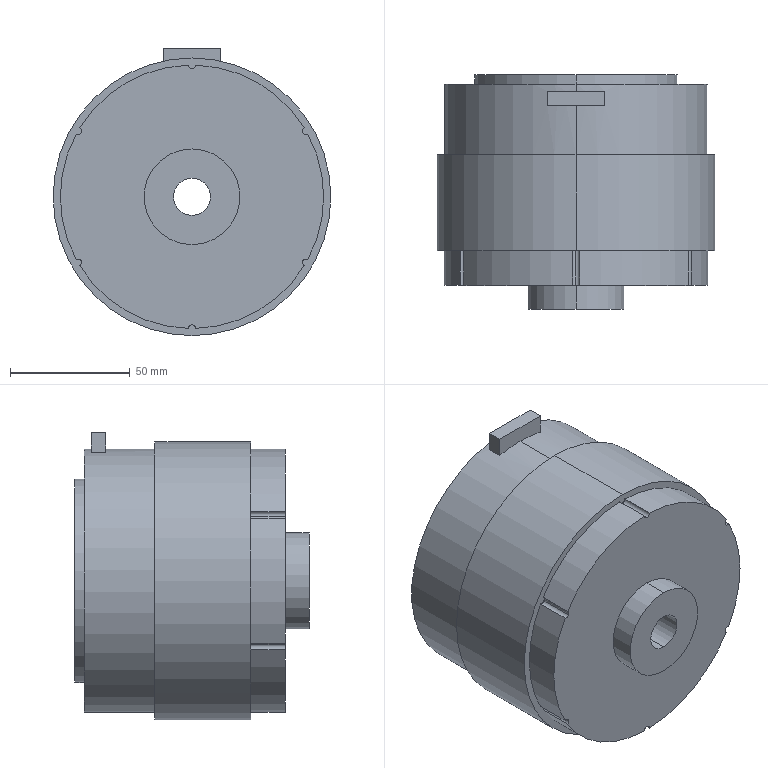Part | STEP file | 1 solid | 45 faces | box 116 x 98 x 120 mm | volume 586421 mm3 | cylinder 32 | plane 13 | commonest cylinder face diameters 3 x12 110 x8 15.5 x2 40 x2 68 x2 69 x2